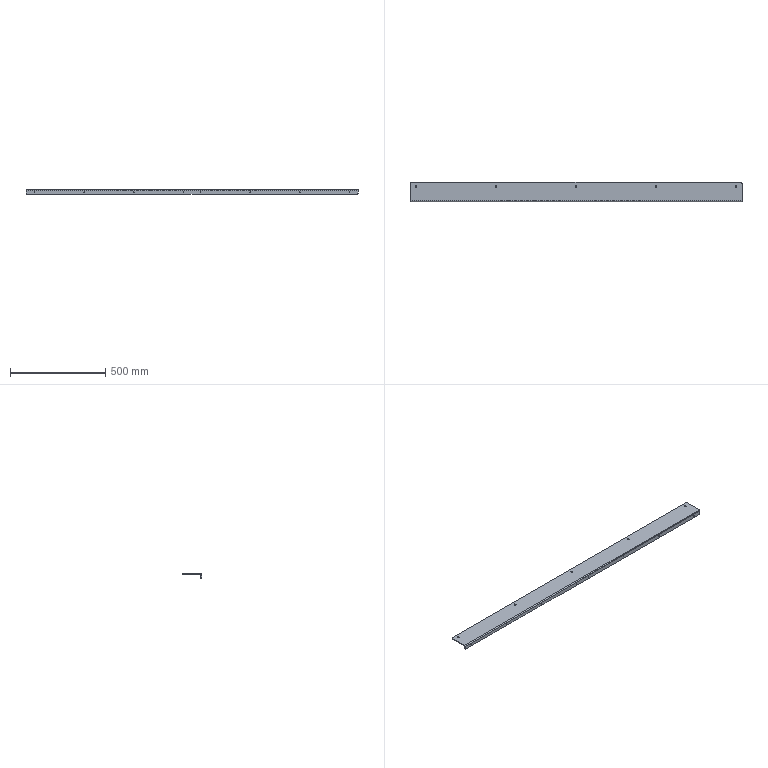Part | SolidWorks | features BaseBody 1 | 1 solid | 54 faces | box 1740 x 100 x 24 mm | volume 825026 mm3 | cylinder 32 | plane 22 | commonest cylinder face diameters 4.2 x16 7 x10 10 x4 1.473 x1 9.473 x1